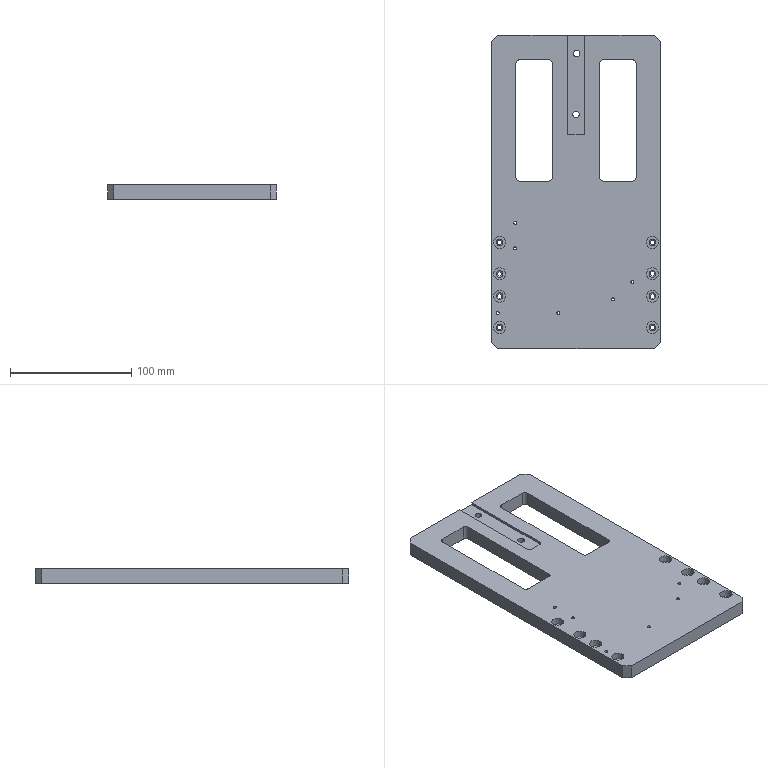Part | SolidWorks | features HoleWzd 4, Cut 2, Fillet 2, Chamfer 1, Extrusion 1 | 1 solid | 110 faces | box 139 x 258 x 12 mm | volume 349365 mm3 | cylinder 62 | plane 32 | cone 16 | commonest cylinder face diameters 5.5 x20 10 x20 2.5 x12 6 x8 4 x2